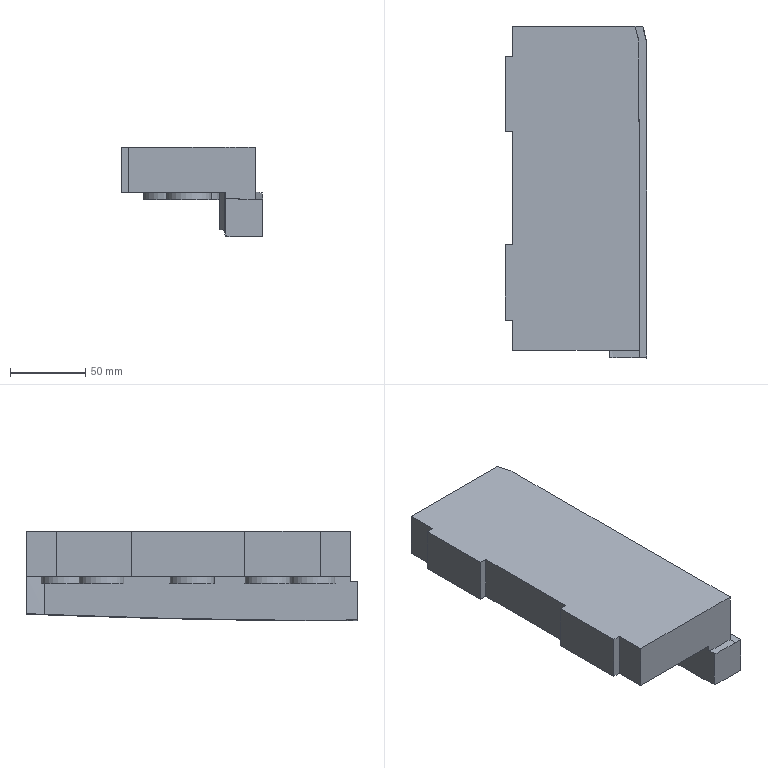Part | NX | features solid 2 | 1 solid | 34 faces | box 93.985 x 220 x 59.615 mm | volume 724597 mm3 | plane 18 | spline 11 | cylinder 5 | commonest cylinder face diameters 30 x5